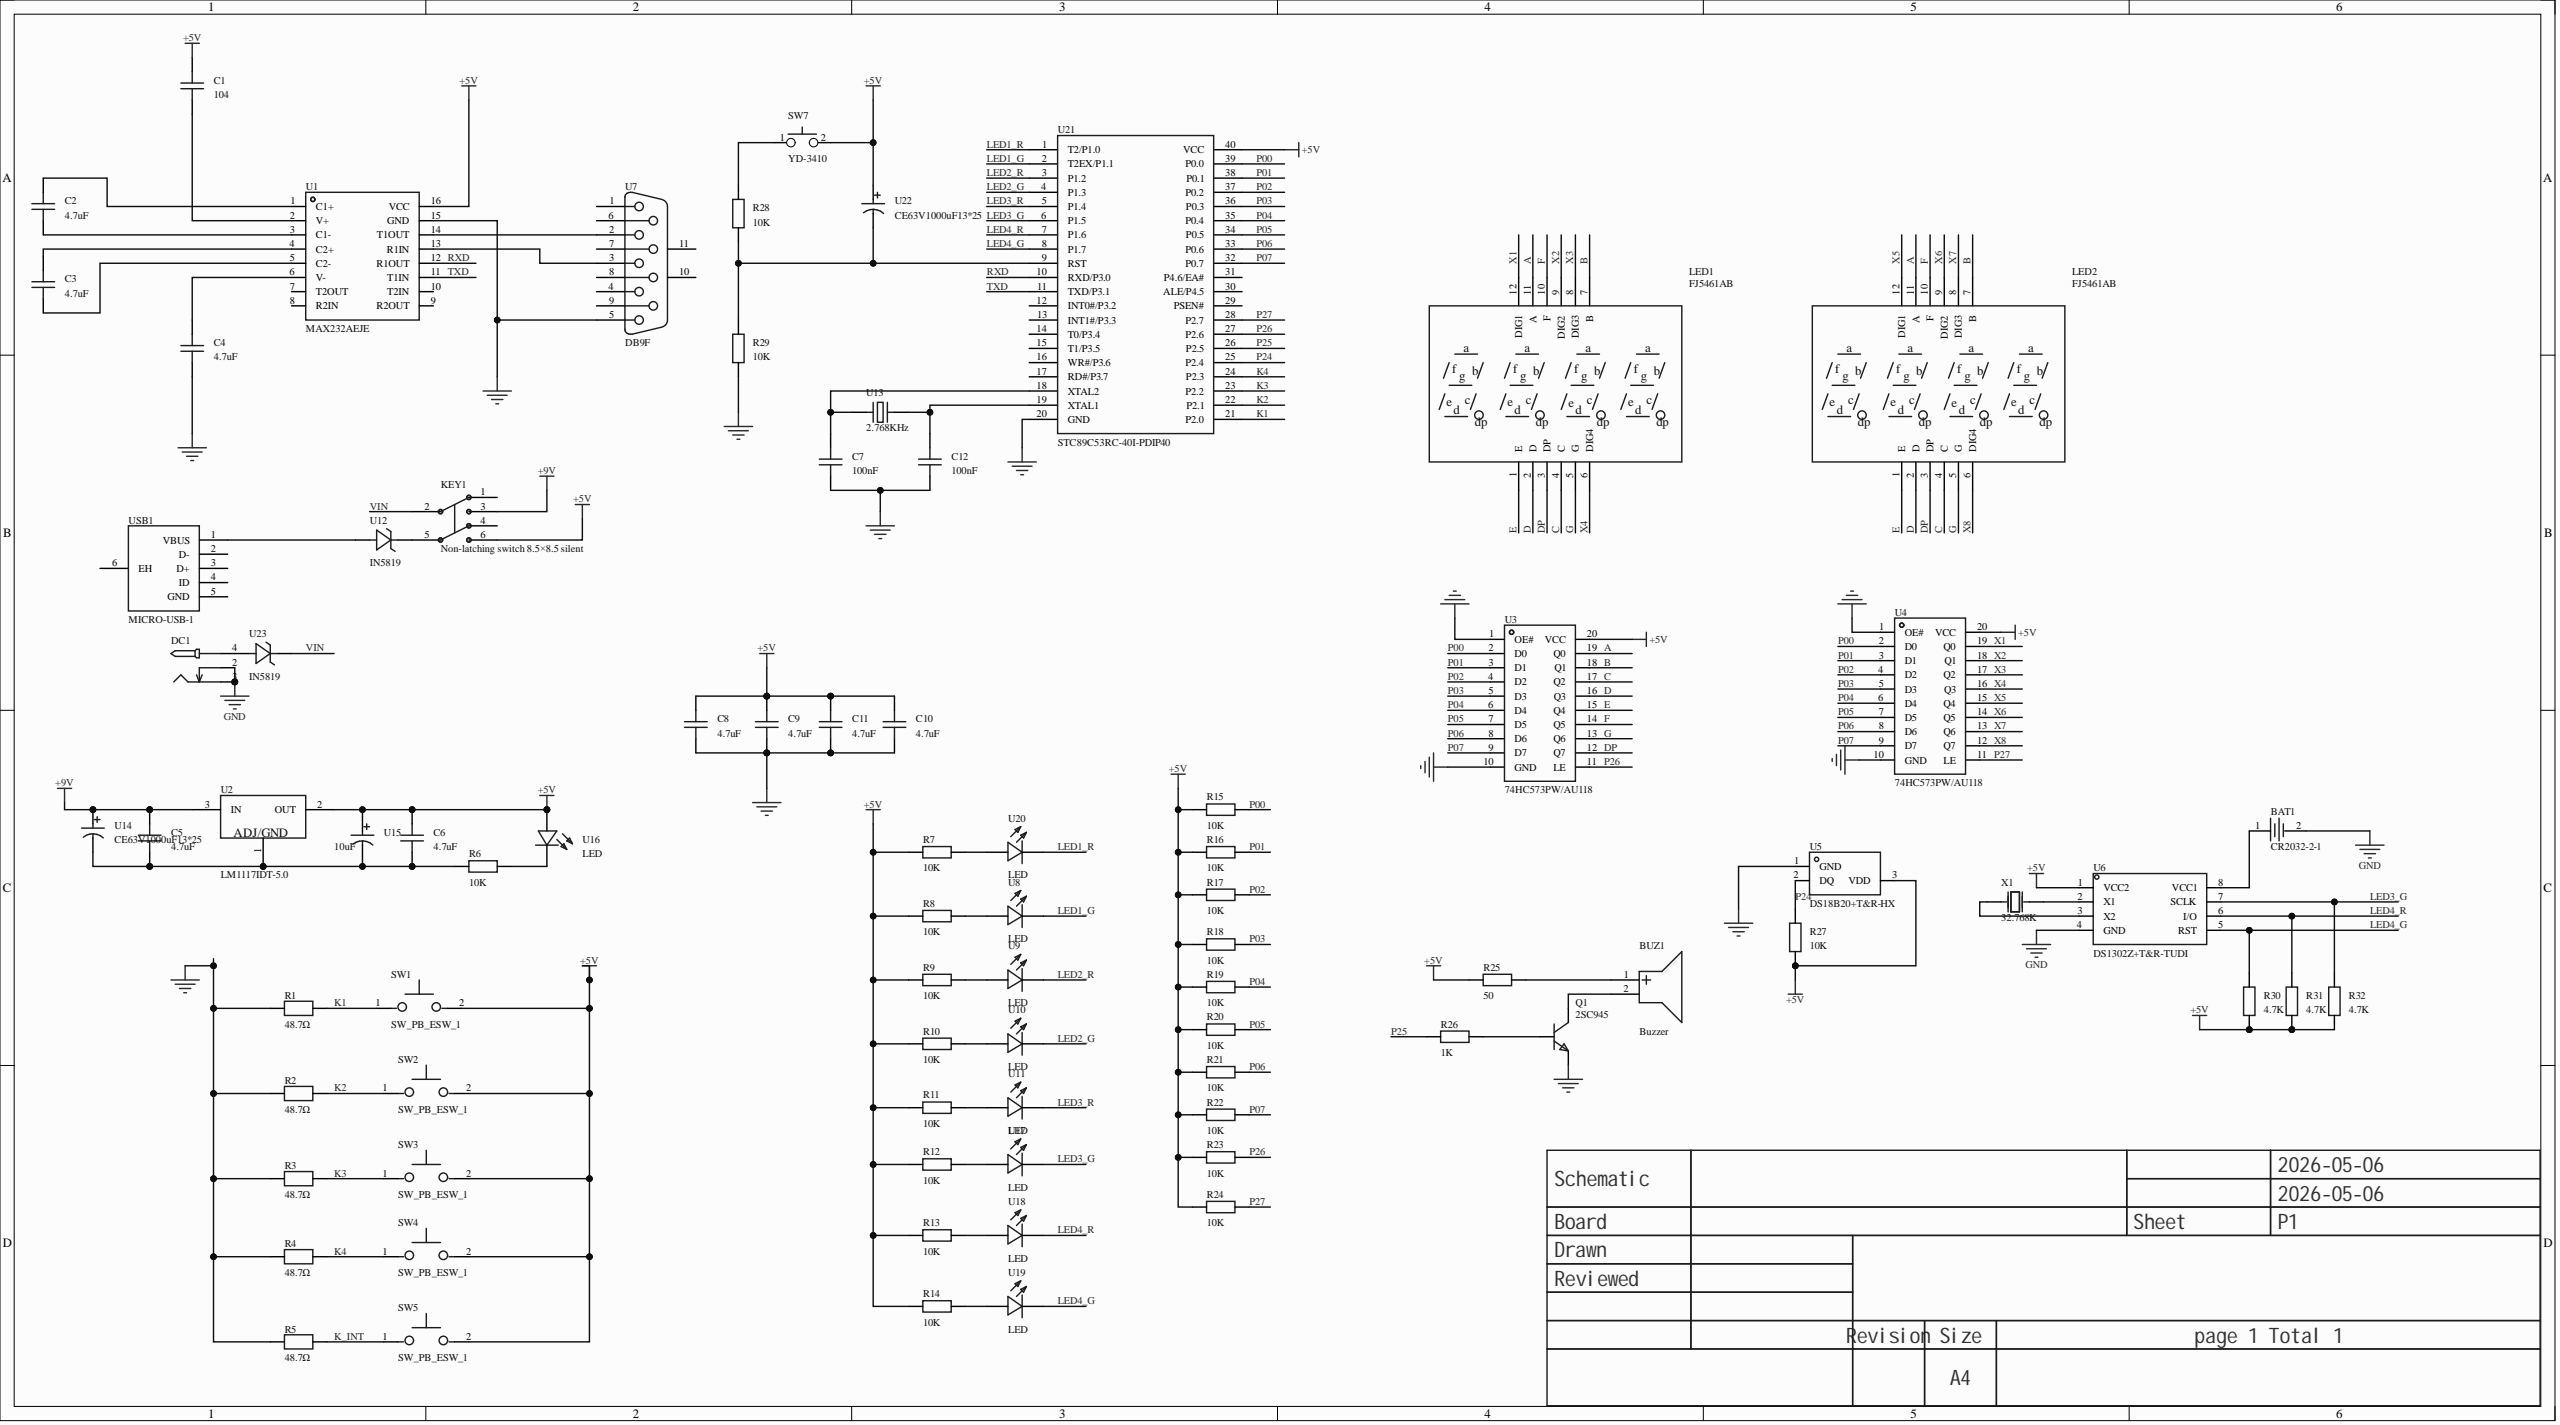Circuit board | Altium Designer | 82 parts | 78 nets
Bill of materials:
Comment,Description,Designator,Footprint,LibRef,Quantity
"CR2032-2-1","","BAT1","BAT-TH_CR2032-2-1","CR2032-2-1","1"
"Buzzer","","BUZ1","BUZ-TH_BD9.0-P5.00-D0.6-FD","蜂鸣器","1"
"104","Capacitance: 4.7uF; tolerance: ±10%; rated voltage: 10V; temperature coefficient: X5R;","C1","C0603","GRM188R61A475KAAJD","1"
"4.7uF","Capacitance: 4.7uF; tolerance: ±10%; rated voltage: 10V; temperature coefficient: X5R;","C2, C3, C4, C5, C6, C8, C9, C10, C11","C0603","GRM188R61A475KAAJD","9"
"100nF","","C7, C12","C0603","CAP_0603","2"
"","","DC1","DC-2.0","DC-005_2.0","1"
"Non-latching switch 8.5×8.5 silent","6 pins, 8.5×8.5","KEY1","SW-TH_6P-L8.5-W8.5-P2.54","无自锁开关 8.5×8.5 无声","1"
"FJ5461AB","","LED1, LED2","LED-SEG-TH_12P-L50.4-W19.0-P2.54-S15.24-BL","FJ5461AB","2"
"2SC945","","Q1","TO-92-3_L4.9-W3.7-P1.27-L","2SC945","1"
"48.7Ω","Resistor type: thick film resistor; resistance: 48.7Ω; tolerance: ±1%; power: 100mW; working voltage: 75V; temperature coefficient: ±100ppm/?;","R1, R2, R3, R4, R5","R0603","FRC0603F48R7TS","5"
"10K","","R6, R7, R8, R9, R10, R11, R12, R13, R14, R15, R16, R17, R18, R19, R20, R21, R22, R23, R24, R27, R28, R29","R0603","Res_0603","22"
"50","","R25","R0603","Res_0603","1"
"1K","","R26","R0603","Res_0603","1"
"4.7K","","R30, R31, R32","R0603","Res_0603","3"
"SW_PB_ESW_1","","SW1, SW2, SW3, SW4, SW5","KEY-SMD_L6.1-W3.8-LS8.0","SW_PB_ESW_1","5"
"YD-3410","","SW7","SW-SMD_L3.9-W2.9-LS4.8-EH-A","YD-3410","1"
"MAX232AEJE","Type: transceiver; data rate: 120Kbps;","U1","PDIP-16_L19.3-W6.5-P2.54-LS7.6-BL","MAX232AEJE","1"
"LM1117IDT-5.0","Output type: fixed; max input voltage: 15V; output voltage: 5V; max output current: 800mA; PSRR: 75dB@(120Hz); output polarity: positive;","U2","TO-252-2_L6.6-W6.1-P4.57-LS9.7-BR-CW","LM1117IDT-5.0","1"
"74HC573PW/AU118","","U3, U4","TSSOP-20_L6.5-W4.4-P0.65-LS6.4-BL","74HC573PW/AU118","2"
"DS18B20+T&R-HX","","U5","TO-92-3_L5.1-W4.1-P1.27-L-1","DS18B20+T&R-HX","1"
"DS1302Z+T&R-TUDI","Real-time clock (RTC)","U6","SOIC-8_L4.9-W3.9-P1.27-LS6.0-BL","DS1302Z+T&R-TUDI","1"
"DB9F","","U7","DB9-TH_DB9F_C9900018961","DB9F","1"
"LED","","U8, U9, U10, U11, U16, U17, U18, U19, U20","LED-TH_BD4.0-P2.54-FD_RED","LED","9"
"IN5819","","U12, U23","SOD-123_L2.7-W1.7-LS3.8-RD","IN5819_C9900008333","2"
"2.768KHz","","U13","CRYSTAL-SMD_L3.2-W1.5-1","2.768KHz","1"
"CE63V1000uF13*25","","U14, U22","CAP-TH_BD13.0-P5.00-D0.6-FD","CE63V1000uF13*25","2"
"10uF","","U15","CAP-TH_BD13.0-P5.00-D0.6-FD","CE63V1000uF13*25","1"
"STC89C53RC-40I-PDIP40","CPU core: 51 family;","U21","DIP-40_L52.0-W13.7-P2.54-LS15.2-BL","STC89C53RC-40I-PDIP40","1"
"MICRO-USB-1","","USB1","MICRO-USB-SMD_C9900008946","MICRO-USB-1","1"
"32.768K","","X1","OSC-SMD_L2.0-W1.2","32.768K","1"
Netlist (Protel format):
[
BAT1
BAT-TH_CR2032-2-1
CR2032-2-1



]
[
BUZ1
BUZ-TH_BD9.0-P5.00-D0.6-FD
Buzzer



]
[
C1
C0603
104



]
[
C2
C0603
4.7uF



]
[
C3
C0603
4.7uF



]
[
C4
C0603
4.7uF



]
[
C5
C0603
4.7uF



]
[
C6
C0603
4.7uF



]
[
C7
C0603
100nF



]
[
C8
C0603
4.7uF



]
[
C9
C0603
4.7uF



]
[
C10
C0603
4.7uF



]
[
C11
C0603
4.7uF



]
[
C12
C0603
100nF



]
[
DC1
DC-2.0




]
[
KEY1
SW-TH_6P-L8.5-W8.5-P2.54
Non-latching switch 8.5×8.5 silent



]
[
LED1
LED-SEG-TH_12P-L50.4-W19.0-P2.54-S15.24-BL
FJ5461AB



]
[
LED2
LED-SEG-TH_12P-L50.4-W19.0-P2.54-S15.24-BL
FJ5461AB



]
[
Q1
TO-92-3_L4.9-W3.7-P1.27-L
2SC945



]
[
R1
R0603
48.7Ω



]
[
R2
R0603
48.7Ω



]
[
R3
R0603
48.7Ω



]
[
R4
R0603
48.7Ω



]
[
R5
R0603
48.7Ω



]
[
R6
R0603
10K



]
[
R7
R0603
10K



]
[
R8
R0603
10K



]
[
R9
R0603
10K



]
[
R10
R0603
10K



]
[
R11
R0603
10K



]
[
R12
R0603
10K



]
[
R13
R0603
10K



]
[
R14
R0603
10K



]
[
R15
R0603
10K



]
[
R16
R0603
10K



]
[
R17
R0603
10K



]
[
R18
R0603
10K



]
[
R19
R0603
10K



]
[
R20
R0603
10K



]
[
R21
R0603
10K



]
[
R22
R0603
10K



]
[
R23
R0603
10K



]
[
R24
R0603
10K



]
[
R25
R0603
50



]
[
R26
R0603
1K



]
[
R27
R0603
10K



]
[
R28
R0603
10K



]
[
R29
R0603
10K



]
[
R30
R0603
4.7K



]
[
R31
R0603
4.7K



]
[
R32
R0603
4.7K



]
[
SW1
KEY-SMD_L6.1-W3.8-LS8.0
SW_PB_ESW_1



]
[
SW2
KEY-SMD_L6.1-W3.8-LS8.0
SW_PB_ESW_1



]
[
SW3
KEY-SMD_L6.1-W3.8-LS8.0
SW_PB_ESW_1



]
[
SW4
KEY-SMD_L6.1-W3.8-LS8.0
SW_PB_ESW_1



]
[
SW5
KEY-SMD_L6.1-W3.8-LS8.0
SW_PB_ESW_1



]
[
SW7
SW-SMD_L3.9-W2.9-LS4.8-EH-A
YD-3410



]
[
U1
PDIP-16_L19.3-W6.5-P2.54-LS7.6-BL
MAX232AEJE



]
[
U2
TO-252-2_L6.6-W6.1-P4.57-LS9.7-BR-CW
LM1117IDT-5.0



]
[
U3
TSSOP-20_L6.5-W4.4-P0.65-LS6.4-BL
74HC573PW/AU118



]
[
U4
TSSOP-20_L6.5-W4.4-P0.65-LS6.4-BL
74HC573PW/AU118



]
[
U5
TO-92-3_L5.1-W4.1-P1.27-L-1
DS18B20+T&R-HX



]
[
U6
SOIC-8_L4.9-W3.9-P1.27-LS6.0-BL
DS1302Z+T&R-TUDI



]
[
U7
DB9-TH_DB9F_C9900018961
DB9F



]
[
U8
LED-TH_BD4.0-P2.54-FD_RED
LED



]
[
U9
LED-TH_BD4.0-P2.54-FD_RED
LED



]
[
U10
LED-TH_BD4.0-P2.54-FD_RED
LED



]
[
U11
LED-TH_BD4.0-P2.54-FD_RED
LED



]
[
U12
SOD-123_L2.7-W1.7-LS3.8-RD
IN5819



]
[
U13
CRYSTAL-SMD_L3.2-W1.5-1
2.768KHz



]
[
U14
CAP-TH_BD13.0-P5.00-D0.6-FD
CE63V1000uF13*25



]
[
U15
CAP-TH_BD13.0-P5.00-D0.6-FD
10uF



]
[
U16
LED-TH_BD4.0-P2.54-FD_RED
LED



]
[
U17
LED-TH_BD4.0-P2.54-FD_RED
LED



]
[
U18
LED-TH_BD4.0-P2.54-FD_RED
LED



]
[
U19
LED-TH_BD4.0-P2.54-FD_RED
LED



]
[
U20
LED-TH_BD4.0-P2.54-FD_RED
LED



]
[
U21
DIP-40_L52.0-W13.7-P2.54-LS15.2-BL
STC89C53RC-40I-PDIP40



]
[
U22
CAP-TH_BD13.0-P5.00-D0.6-FD
CE63V1000uF13*25



]
[
U23
SOD-123_L2.7-W1.7-LS3.8-RD
IN5819



]
[
USB1
MICRO-USB-SMD_C9900008946
MICRO-USB-1



]
[
X1
OSC-SMD_L2.0-W1.2
32.768K



]
(
X8
LED2-6
U4-12
)
(
X7
LED2-8
U4-13
)
(
X6
LED2-9
U4-14
)
(
X5
LED2-12
U4-15
)
(
X4
LED1-6
U4-16
)
(
X3
LED1-8
U4-17
)
(
X2
LED1-9
U4-18
)
(
X1
LED1-12
U4-19
)
(
VIN
KEY1-2
U23-1
)
(
TXD
U1-11
U21-11
)
(
RXD
U1-12
U21-10
)
(
P27
R24-2
U4-11
U21-28
)
(
P26
R23-2
U3-11
U21-27
)
(
P25
R26-1
U21-26
)
(
P24
R27-2
U5-2
U21-25
)
(
P07
R22-2
U3-9
U4-9
U21-32
)
(
P06
R21-2
U3-8
U4-8
U21-33
)
(
P05
R20-2
U3-7
U4-7
U21-34
)
(
P04
R19-2
U3-6
U4-6
U21-35
)
(
P03
R18-2
U3-5
U4-5
U21-36
)
(
P02
R17-2
U3-4
U4-4
U21-37
)
(
P01
R16-2
U3-3
U4-3
U21-38
)
(
P00
R15-2
U3-2
U4-2
U21-39
)
(
NetU12_2
U12-2
USB1-1
)
(
NetU6_3
U6-3
X1-1
)
(
NetU6_2
U6-2
X1-2
)
(
NetU1_14
U1-14
U7-2
)
(
NetU1_13
U1-13
U7-3
)
(
NetR28_2
R28-2
SW7-1
)
(
NetR28_1
R28-1
R29-2
U21-9
U22-2
)
(
NetR14_2
R14-2
U19-1
)
(
NetR13_2
R13-2
U18-1
)
(
NetR12_2
R12-2
U17-1
)
(
NetR11_2
R11-2
U11-1
)
(
NetR10_2
R10-2
U10-1
)
(
NetR9_2
R9-2
U9-1
)
(
NetR8_2
R8-2
U8-1
)
(
NetR7_2
R7-2
U20-1
)
(
NetR6_2
R6-2
U16-2
)
(
NetQ1_3
Q1-3
R26-2
)
(
NetKEY1_5
KEY1-5
U12-1
)
(
NetDC1_4
DC1-4
U23-2
)
(
NetC12_2
C12-2
U13-2
U21-19
)
(
NetC7_2
C7-2
U13-1
U21-18
)
(
NetC5_1
C5-1
C6-1
R6-1
U2-1
U14-2
U15-2
)
(
NetC4_2
C4-2
U1-6
)
(
NetC3_2
C3-2
U1-4
)
(
NetC3_1
C3-1
U1-5
)
(
NetC2_2
C2-2
U1-1
)
(
NetC2_1
C2-1
U1-3
)
(
NetC1_1
C1-1
U1-2
)
(
NetBUZ1_2
BUZ1-2
Q1-2
)
(
NetBUZ1_1
BUZ1-1
R25-2
)
(
NetBAT1_1
BAT1-1
U6-8
)
(
LED4_R
R31-2
U6-6
U18-2
U21-7
)
(
LED4_G
R30-2
U6-5
U19-2
U21-8
)
(
LED3_R
U11-2
U21-5
)
(
LED3_G
R32-2
U6-7
U17-2
U21-6
)
(
LED2_R
U9-2
U21-3
)
(
LED2_G
U10-2
U21-4
)
(
LED1_R
U20-2
U21-1
)
(
LED1_G
U8-2
U21-2
)
(
K_INT
R5-2
SW5-1
)
(
K4
R4-2
SW4-1
U21-24
)
(
K3
R3-2
SW3-1
U21-23
)
(
K2
R2-2
SW2-1
U21-22
)
(
K1
R1-2
SW1-1
U21-21
)
(
GND
BAT1-2
C4-1
C7-1
C8-1
C9-1
C10-1
C11-1
C12-1
DC1-2
DC1-3
Q1-1
R1-1
R2-1
R3-1
R4-1
R5-1
R29-1
U1-15
U3-1
U3-10
U4-1
U4-10
U5-1
U6-4
U7-5
U21-20
)
(
G
LED1-5
LED2-5
U3-13
)
(
F
LED1-10
LED2-10
U3-14
)
(
E
LED1-1
LED2-1
U3-15
)
(
DP
LED1-3
LED2-3
U3-12
)
(
D
LED1-2
LED2-2
U3-16
)
(
C
LED1-4
LED2-4
U3-17
)
(
B
LED1-7
LED2-7
U3-18
)
(
A
LED1-11
LED2-11
U3-19
)
(
+9V
C5-2
KEY1-3
U2-3
U14-1
)
(
+5V
C1-2
C6-2
C8-2
C9-2
C10-2
C11-2
KEY1-6
R7-1
R8-1
R9-1
R10-1
R11-1
R12-1
R13-1
R14-1
R15-1
R16-1
R17-1
R18-1
R19-1
R20-1
R21-1
R22-1
R23-1
R24-1
R25-1
R27-1
R30-1
R31-1
R32-1
SW1-2
SW2-2
SW3-2
SW4-2
SW5-2
SW7-2
U1-16
U2-2
U3-20
U4-20
U5-3
U6-1
U15-1
U16-1
U21-40
U22-1
)